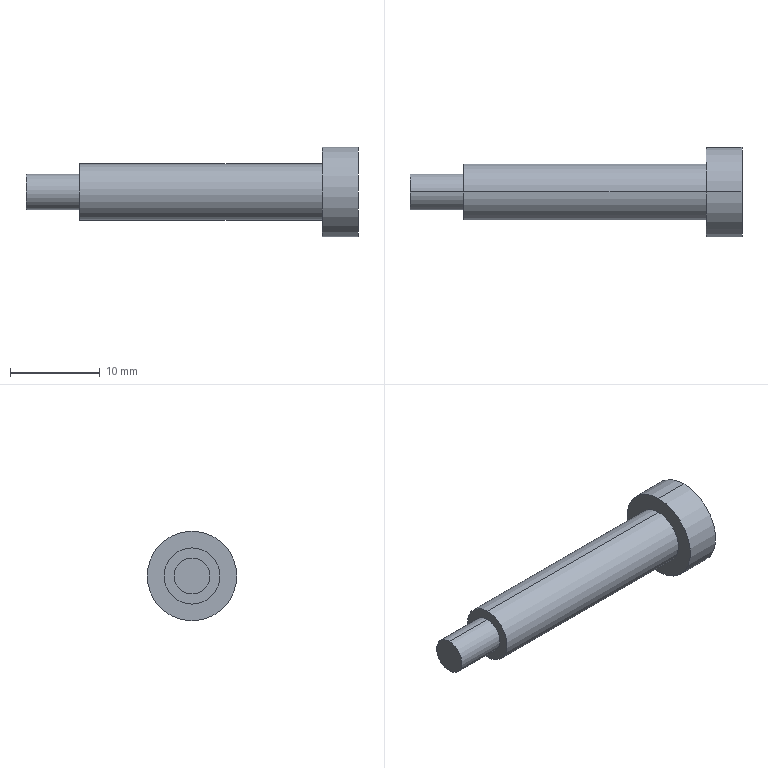Part | SolidWorks | features Revolution 1 | 1 solid | 10 faces | box 37 x 10 x 10 mm | volume 1218 mm3 | cylinder 6 | plane 4 | commonest cylinder face diameters 4 x2 6.25 x2 10 x2
STEP:
#1=CARTESIAN_POINT('',(0.7574,0.,0.1969));
#2=VERTEX_POINT('',#1);
#3=CARTESIAN_POINT('',(0.7574,0.,-0.1969));
#4=VERTEX_POINT('',#3);
#5=CARTESIAN_POINT('',(0.7574,0.,0.));
#6=DIRECTION('',(-1.,0.,0.));
#7=DIRECTION('',(0.,0.,1.));
#8=AXIS2_PLACEMENT_3D('',#5,#6,#7);
#9=CIRCLE('',#8,0.1969);
#10=EDGE_CURVE('',#2,#4,#9,.T.);
#11=ORIENTED_EDGE('',*,*,#10,.T.);
#12=CARTESIAN_POINT('',(0.6,0.,-0.1969));
#13=VERTEX_POINT('',#12);
#14=CARTESIAN_POINT('',(-1.049,0.,-0.1969));
#15=DIRECTION('',(-1.,0.,0.));
#16=VECTOR('',#15,39.37);
#17=LINE('',#14,#16);
#18=EDGE_CURVE('',#4,#13,#17,.T.);
#19=ORIENTED_EDGE('',*,*,#18,.T.);
#20=CARTESIAN_POINT('',(0.6,0.,0.1969));
#21=VERTEX_POINT('',#20);
#22=CARTESIAN_POINT('',(0.6,0.,0.));
#23=DIRECTION('',(-1.,0.,0.));
#24=DIRECTION('',(0.,0.,1.));
#25=AXIS2_PLACEMENT_3D('',#22,#23,#24);
#26=CIRCLE('',#25,0.1969);
#27=EDGE_CURVE('',#21,#13,#26,.T.);
#28=ORIENTED_EDGE('',*,*,#27,.F.);
#29=CARTESIAN_POINT('',(-1.049,0.,0.1969));
#30=DIRECTION('',(-1.,0.,0.));
#31=VECTOR('',#30,39.37);
#32=LINE('',#29,#31);
#33=EDGE_CURVE('',#2,#21,#32,.T.);
#34=ORIENTED_EDGE('',*,*,#33,.F.);
#35=EDGE_LOOP('',(#11,#19,#28,#34));
#36=FACE_OUTER_BOUND('',#35,.T.);
#37=CARTESIAN_POINT('',(-1.049,0.,0.));
#38=DIRECTION('',(-1.,0.,0.));
#39=DIRECTION('',(0.,0.,1.));
#40=AXIS2_PLACEMENT_3D('',#37,#38,#39);
#41=CYLINDRICAL_SURFACE('',#40,0.1969);
#42=ADVANCED_FACE('',(#36),#41,.T.);
#43=CARTESIAN_POINT('',(0.6,0.,0.123));
#44=VERTEX_POINT('',#43);
#45=CARTESIAN_POINT('',(0.6,0.,-0.123));
#46=VERTEX_POINT('',#45);
#47=CARTESIAN_POINT('',(0.6,0.,0.));
#48=DIRECTION('',(-1.,0.,0.));
#49=DIRECTION('',(0.,0.,1.));
#50=AXIS2_PLACEMENT_3D('',#47,#48,#49);
#51=CIRCLE('',#50,0.123);
#52=EDGE_CURVE('',#44,#46,#51,.T.);
#53=ORIENTED_EDGE('',*,*,#52,.T.);
#54=CARTESIAN_POINT('',(-0.463,0.,-0.123));
#55=VERTEX_POINT('',#54);
#56=CARTESIAN_POINT('',(-1.049,0.,-0.123));
#57=DIRECTION('',(-1.,0.,0.));
#58=VECTOR('',#57,39.37);
#59=LINE('',#56,#58);
#60=EDGE_CURVE('',#46,#55,#59,.T.);
#61=ORIENTED_EDGE('',*,*,#60,.T.);
#62=CARTESIAN_POINT('',(-0.463,0.,0.123));
#63=VERTEX_POINT('',#62);
#64=CARTESIAN_POINT('',(-0.463,0.,0.));
#65=DIRECTION('',(-1.,0.,0.));
#66=DIRECTION('',(0.,0.,1.));
#67=AXIS2_PLACEMENT_3D('',#64,#65,#66);
#68=CIRCLE('',#67,0.123);
#69=EDGE_CURVE('',#63,#55,#68,.T.);
#70=ORIENTED_EDGE('',*,*,#69,.F.);
#71=CARTESIAN_POINT('',(-1.049,0.,0.123));
#72=DIRECTION('',(-1.,0.,0.));
#73=VECTOR('',#72,39.37);
#74=LINE('',#71,#73);
#75=EDGE_CURVE('',#44,#63,#74,.T.);
#76=ORIENTED_EDGE('',*,*,#75,.F.);
#77=EDGE_LOOP('',(#53,#61,#70,#76));
#78=FACE_OUTER_BOUND('',#77,.T.);
#79=CARTESIAN_POINT('',(-1.049,0.,0.));
#80=DIRECTION('',(-1.,0.,0.));
#81=DIRECTION('',(0.,0.,1.));
#82=AXIS2_PLACEMENT_3D('',#79,#80,#81);
#83=CYLINDRICAL_SURFACE('',#82,0.123);
#84=ADVANCED_FACE('',(#78),#83,.T.);
#85=CARTESIAN_POINT('',(-0.463,0.,0.07874));
#86=VERTEX_POINT('',#85);
#87=CARTESIAN_POINT('',(-0.463,0.,-0.07874));
#88=VERTEX_POINT('',#87);
#89=CARTESIAN_POINT('',(-0.463,0.,0.));
#90=DIRECTION('',(-1.,0.,0.));
#91=DIRECTION('',(0.,0.,1.));
#92=AXIS2_PLACEMENT_3D('',#89,#90,#91);
#93=CIRCLE('',#92,0.07874);
#94=EDGE_CURVE('',#86,#88,#93,.T.);
#95=ORIENTED_EDGE('',*,*,#94,.T.);
#96=CARTESIAN_POINT('',(-0.6992,0.,-0.07874));
#97=VERTEX_POINT('',#96);
#98=CARTESIAN_POINT('',(-1.049,0.,-0.07874));
#99=DIRECTION('',(-1.,0.,0.));
#100=VECTOR('',#99,39.37);
#101=LINE('',#98,#100);
#102=EDGE_CURVE('',#88,#97,#101,.T.);
#103=ORIENTED_EDGE('',*,*,#102,.T.);
#104=CARTESIAN_POINT('',(-0.6992,0.,0.07874));
#105=VERTEX_POINT('',#104);
#106=CARTESIAN_POINT('',(-0.6992,0.,0.));
#107=DIRECTION('',(-1.,0.,0.));
#108=DIRECTION('',(0.,0.,1.));
#109=AXIS2_PLACEMENT_3D('',#106,#107,#108);
#110=CIRCLE('',#109,0.07874);
#111=EDGE_CURVE('',#105,#97,#110,.T.);
#112=ORIENTED_EDGE('',*,*,#111,.F.);
#113=CARTESIAN_POINT('',(-1.049,0.,0.07874));
#114=DIRECTION('',(-1.,0.,0.));
#115=VECTOR('',#114,39.37);
#116=LINE('',#113,#115);
#117=EDGE_CURVE('',#86,#105,#116,.T.);
#118=ORIENTED_EDGE('',*,*,#117,.F.);
#119=EDGE_LOOP('',(#95,#103,#112,#118));
#120=FACE_OUTER_BOUND('',#119,.T.);
#121=CARTESIAN_POINT('',(-1.049,0.,0.));
#122=DIRECTION('',(-1.,0.,0.));
#123=DIRECTION('',(0.,0.,1.));
#124=AXIS2_PLACEMENT_3D('',#121,#122,#123);
#125=CYLINDRICAL_SURFACE('',#124,0.07874);
#126=ADVANCED_FACE('',(#120),#125,.T.);
#127=ORIENTED_EDGE('',*,*,#111,.T.);
#128=CARTESIAN_POINT('',(-0.6992,0.,0.));
#129=DIRECTION('',(-1.,0.,0.));
#130=DIRECTION('',(0.,0.,1.));
#131=AXIS2_PLACEMENT_3D('',#128,#129,#130);
#132=CIRCLE('',#131,0.07874);
#133=EDGE_CURVE('',#97,#105,#132,.T.);
#134=ORIENTED_EDGE('',*,*,#133,.T.);
#135=EDGE_LOOP('',(#127,#134));
#136=FACE_OUTER_BOUND('',#135,.T.);
#137=CARTESIAN_POINT('',(-0.6992,0.,0.));
#138=DIRECTION('',(-1.,0.,0.));
#139=DIRECTION('',(0.,0.,1.));
#140=AXIS2_PLACEMENT_3D('',#137,#138,#139);
#141=PLANE('',#140);
#142=ADVANCED_FACE('',(#136),#141,.T.);
#143=ORIENTED_EDGE('',*,*,#102,.F.);
#144=CARTESIAN_POINT('',(-0.463,0.,0.));
#145=DIRECTION('',(-1.,0.,0.));
#146=DIRECTION('',(0.,0.,1.));
#147=AXIS2_PLACEMENT_3D('',#144,#145,#146);
#148=CIRCLE('',#147,0.07874);
#149=EDGE_CURVE('',#88,#86,#148,.T.);
#150=ORIENTED_EDGE('',*,*,#149,.T.);
#151=ORIENTED_EDGE('',*,*,#117,.T.);
#152=ORIENTED_EDGE('',*,*,#133,.F.);
#153=EDGE_LOOP('',(#143,#150,#151,#152));
#154=FACE_OUTER_BOUND('',#153,.T.);
#155=CARTESIAN_POINT('',(-1.049,0.,0.));
#156=DIRECTION('',(-1.,0.,0.));
#157=DIRECTION('',(0.,0.,1.));
#158=AXIS2_PLACEMENT_3D('',#155,#156,#157);
#159=CYLINDRICAL_SURFACE('',#158,0.07874);
#160=ADVANCED_FACE('',(#154),#159,.T.);
#161=ORIENTED_EDGE('',*,*,#69,.T.);
#162=CARTESIAN_POINT('',(-0.463,0.,0.));
#163=DIRECTION('',(-1.,0.,0.));
#164=DIRECTION('',(0.,0.,1.));
#165=AXIS2_PLACEMENT_3D('',#162,#163,#164);
#166=CIRCLE('',#165,0.123);
#167=EDGE_CURVE('',#55,#63,#166,.T.);
#168=ORIENTED_EDGE('',*,*,#167,.T.);
#169=EDGE_LOOP('',(#161,#168));
#170=FACE_OUTER_BOUND('',#169,.T.);
#171=ORIENTED_EDGE('',*,*,#94,.F.);
#172=ORIENTED_EDGE('',*,*,#149,.F.);
#173=EDGE_LOOP('',(#171,#172));
#174=FACE_BOUND('',#173,.T.);
#175=CARTESIAN_POINT('',(-0.463,-0.07874,0.));
#176=DIRECTION('',(-1.,0.,0.));
#177=DIRECTION('',(0.,0.,1.));
#178=AXIS2_PLACEMENT_3D('',#175,#176,#177);
#179=PLANE('',#178);
#180=ADVANCED_FACE('',(#170,#174),#179,.T.);
#181=ORIENTED_EDGE('',*,*,#60,.F.);
#182=CARTESIAN_POINT('',(0.6,0.,0.));
#183=DIRECTION('',(-1.,0.,0.));
#184=DIRECTION('',(0.,0.,1.));
#185=AXIS2_PLACEMENT_3D('',#182,#183,#184);
#186=CIRCLE('',#185,0.123);
#187=EDGE_CURVE('',#46,#44,#186,.T.);
#188=ORIENTED_EDGE('',*,*,#187,.T.);
#189=ORIENTED_EDGE('',*,*,#75,.T.);
#190=ORIENTED_EDGE('',*,*,#167,.F.);
#191=EDGE_LOOP('',(#181,#188,#189,#190));
#192=FACE_OUTER_BOUND('',#191,.T.);
#193=CARTESIAN_POINT('',(-1.049,0.,0.));
#194=DIRECTION('',(-1.,0.,0.));
#195=DIRECTION('',(0.,0.,1.));
#196=AXIS2_PLACEMENT_3D('',#193,#194,#195);
#197=CYLINDRICAL_SURFACE('',#196,0.123);
#198=ADVANCED_FACE('',(#192),#197,.T.);
#199=ORIENTED_EDGE('',*,*,#27,.T.);
#200=CARTESIAN_POINT('',(0.6,0.,0.));
#201=DIRECTION('',(-1.,0.,0.));
#202=DIRECTION('',(0.,0.,1.));
#203=AXIS2_PLACEMENT_3D('',#200,#201,#202);
#204=CIRCLE('',#203,0.1969);
#205=EDGE_CURVE('',#13,#21,#204,.T.);
#206=ORIENTED_EDGE('',*,*,#205,.T.);
#207=EDGE_LOOP('',(#199,#206));
#208=FACE_OUTER_BOUND('',#207,.T.);
#209=ORIENTED_EDGE('',*,*,#52,.F.);
#210=ORIENTED_EDGE('',*,*,#187,.F.);
#211=EDGE_LOOP('',(#209,#210));
#212=FACE_BOUND('',#211,.T.);
#213=CARTESIAN_POINT('',(0.6,-0.123,0.));
#214=DIRECTION('',(-1.,0.,0.));
#215=DIRECTION('',(0.,0.,1.));
#216=AXIS2_PLACEMENT_3D('',#213,#214,#215);
#217=PLANE('',#216);
#218=ADVANCED_FACE('',(#208,#212),#217,.T.);
#219=ORIENTED_EDGE('',*,*,#18,.F.);
#220=CARTESIAN_POINT('',(0.7574,0.,0.));
#221=DIRECTION('',(-1.,0.,0.));
#222=DIRECTION('',(0.,0.,1.));
#223=AXIS2_PLACEMENT_3D('',#220,#221,#222);
#224=CIRCLE('',#223,0.1969);
#225=EDGE_CURVE('',#4,#2,#224,.T.);
#226=ORIENTED_EDGE('',*,*,#225,.T.);
#227=ORIENTED_EDGE('',*,*,#33,.T.);
#228=ORIENTED_EDGE('',*,*,#205,.F.);
#229=EDGE_LOOP('',(#219,#226,#227,#228));
#230=FACE_OUTER_BOUND('',#229,.T.);
#231=CARTESIAN_POINT('',(-1.049,0.,0.));
#232=DIRECTION('',(-1.,0.,0.));
#233=DIRECTION('',(0.,0.,1.));
#234=AXIS2_PLACEMENT_3D('',#231,#232,#233);
#235=CYLINDRICAL_SURFACE('',#234,0.1969);
#236=ADVANCED_FACE('',(#230),#235,.T.);
#237=ORIENTED_EDGE('',*,*,#10,.F.);
#238=ORIENTED_EDGE('',*,*,#225,.F.);
#239=EDGE_LOOP('',(#237,#238));
#240=FACE_OUTER_BOUND('',#239,.T.);
#241=CARTESIAN_POINT('',(0.7574,-0.1969,0.));
#242=DIRECTION('',(1.,0.,0.));
#243=DIRECTION('',(0.,0.,-1.));
#244=AXIS2_PLACEMENT_3D('',#241,#242,#243);
#245=PLANE('',#244);
#246=ADVANCED_FACE('',(#240),#245,.T.);
#247=CLOSED_SHELL('',(#42,#84,#126,#142,#160,#180,#198,#218,#236,#246));
#248=MANIFOLD_SOLID_BREP('',#247);
#249=CARTESIAN_POINT('',(0.,0.,0.));
#250=DIRECTION('',(0.,0.,1.));
#251=DIRECTION('',(1.,0.,0.));
#252=AXIS2_PLACEMENT_3D('',#249,#250,#251);
#253=(LENGTH_UNIT()NAMED_UNIT(*)SI_UNIT($,.METRE.));
#254=LENGTH_MEASURE_WITH_UNIT(LENGTH_MEASURE(0.0254),#253);
#255=DIMENSIONAL_EXPONENTS(1.,0.,0.,0.,0.,0.,0.);
#256=(CONVERSION_BASED_UNIT('INCH',#254)LENGTH_UNIT()NAMED_UNIT(#255));
#257=UNCERTAINTY_MEASURE_WITH_UNIT(LENGTH_MEASURE(0.00001),#256,'','');
#258=(NAMED_UNIT(*)PLANE_ANGLE_UNIT()SI_UNIT($,.RADIAN.));
#259=(NAMED_UNIT(*)SI_UNIT($,.STERADIAN.)SOLID_ANGLE_UNIT());
#260=(GEOMETRIC_REPRESENTATION_CONTEXT(3)GLOBAL_UNCERTAINTY_ASSIGNED_CONTEXT((#257))GLOBAL_UNIT_ASSIGNED_CONTEXT((#256,#258,#259))REPRESENTATION_CONTEXT('',''));
#261=ADVANCED_BREP_SHAPE_REPRESENTATION('',(#248,#252),#260);